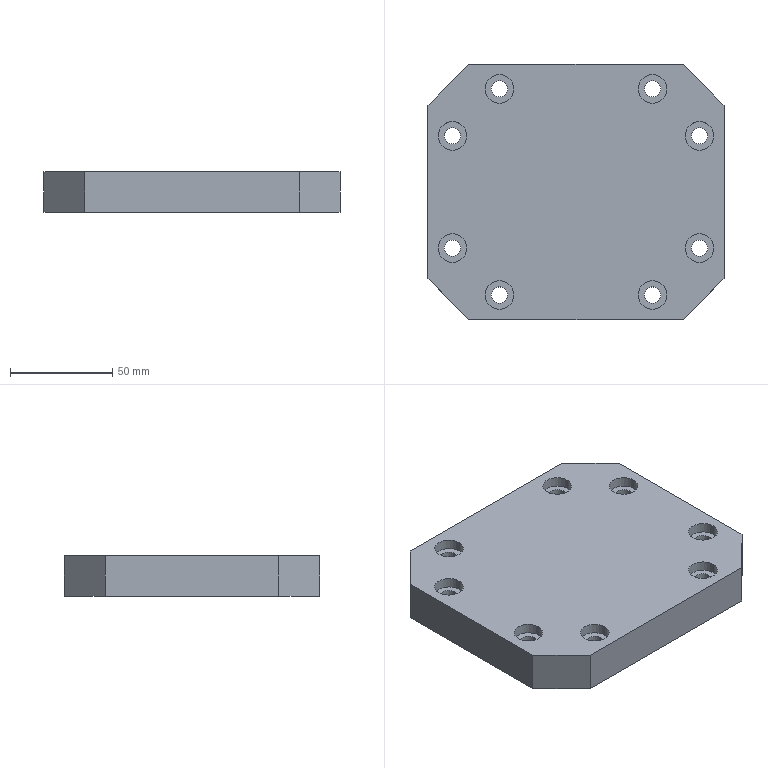Part | SolidWorks | features ICE 4, Chamfer 1, Extrusion 1 | 1 solid | 61 faces | box 145 x 125 x 20 mm | volume 332455 mm3 | cylinder 38 | plane 23 | commonest cylinder face diameters 8 x16 14 x16 5 x6